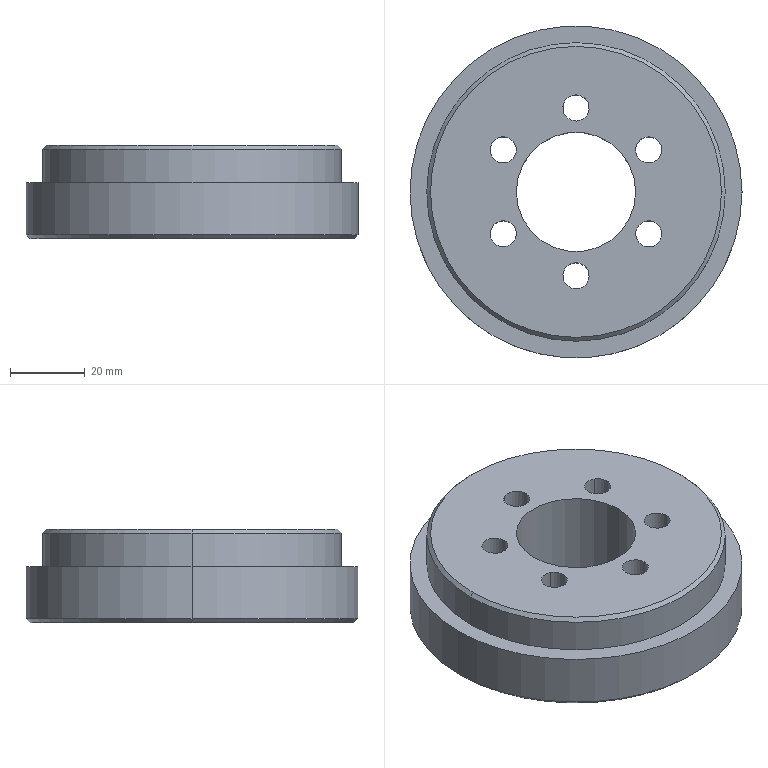Part | SolidWorks | features BaseBody 1 | 1 solid | 25 faces | box 89 x 89 x 25 mm | volume 117440 mm3 | cylinder 18 | cone 4 | plane 3 | commonest cylinder face diameters 7 x12 32 x2 80 x2 89 x2
STEP:
#1=CARTESIAN_POINT('',(17.736,8.219,0.));
#2=VERTEX_POINT('',#1);
#3=CARTESIAN_POINT('',(21.236,14.281,0.));
#4=VERTEX_POINT('',#3);
#5=CARTESIAN_POINT('',(19.486,11.25,0.));
#6=DIRECTION('',(0.,0.,1.));
#7=DIRECTION('',(0.5,0.866,0.));
#8=AXIS2_PLACEMENT_3D('',#5,#6,#7);
#9=CIRCLE('',#8,3.5);
#10=EDGE_CURVE('',#2,#4,#9,.T.);
#11=ORIENTED_EDGE('',*,*,#10,.F.);
#12=CARTESIAN_POINT('',(17.736,8.219,25.));
#13=VERTEX_POINT('',#12);
#14=CARTESIAN_POINT('',(17.736,8.219,0.));
#15=DIRECTION('',(0.,0.,1.));
#16=VECTOR('',#15,1000.);
#17=LINE('',#14,#16);
#18=EDGE_CURVE('',#2,#13,#17,.T.);
#19=ORIENTED_EDGE('',*,*,#18,.T.);
#20=CARTESIAN_POINT('',(21.236,14.281,25.));
#21=VERTEX_POINT('',#20);
#22=CARTESIAN_POINT('',(19.486,11.25,25.));
#23=DIRECTION('',(0.,0.,1.));
#24=DIRECTION('',(0.5,0.866,0.));
#25=AXIS2_PLACEMENT_3D('',#22,#23,#24);
#26=CIRCLE('',#25,3.5);
#27=EDGE_CURVE('',#13,#21,#26,.T.);
#28=ORIENTED_EDGE('',*,*,#27,.T.);
#29=CARTESIAN_POINT('',(21.236,14.281,0.));
#30=DIRECTION('',(0.,0.,1.));
#31=VECTOR('',#30,1000.);
#32=LINE('',#29,#31);
#33=EDGE_CURVE('',#4,#21,#32,.T.);
#34=ORIENTED_EDGE('',*,*,#33,.F.);
#35=EDGE_LOOP('',(#11,#19,#28,#34));
#36=FACE_OUTER_BOUND('',#35,.T.);
#37=CARTESIAN_POINT('',(19.486,11.25,0.));
#38=DIRECTION('',(0.,0.,1.));
#39=DIRECTION('',(0.5,0.866,0.));
#40=AXIS2_PLACEMENT_3D('',#37,#38,#39);
#41=CYLINDRICAL_SURFACE('',#40,3.5);
#42=ADVANCED_FACE('',(#36),#41,.F.);
#43=CARTESIAN_POINT('',(1.75,19.469,0.));
#44=VERTEX_POINT('',#43);
#45=CARTESIAN_POINT('',(-1.75,25.531,0.));
#46=VERTEX_POINT('',#45);
#47=CARTESIAN_POINT('',(0.,22.5,0.));
#48=DIRECTION('',(0.,0.,1.));
#49=DIRECTION('',(-0.5,0.866,0.));
#50=AXIS2_PLACEMENT_3D('',#47,#48,#49);
#51=CIRCLE('',#50,3.5);
#52=EDGE_CURVE('',#44,#46,#51,.T.);
#53=ORIENTED_EDGE('',*,*,#52,.F.);
#54=CARTESIAN_POINT('',(1.75,19.469,25.));
#55=VERTEX_POINT('',#54);
#56=CARTESIAN_POINT('',(1.75,19.469,0.));
#57=DIRECTION('',(0.,0.,1.));
#58=VECTOR('',#57,1000.);
#59=LINE('',#56,#58);
#60=EDGE_CURVE('',#44,#55,#59,.T.);
#61=ORIENTED_EDGE('',*,*,#60,.T.);
#62=CARTESIAN_POINT('',(-1.75,25.531,25.));
#63=VERTEX_POINT('',#62);
#64=CARTESIAN_POINT('',(0.,22.5,25.));
#65=DIRECTION('',(0.,0.,1.));
#66=DIRECTION('',(-0.5,0.866,0.));
#67=AXIS2_PLACEMENT_3D('',#64,#65,#66);
#68=CIRCLE('',#67,3.5);
#69=EDGE_CURVE('',#55,#63,#68,.T.);
#70=ORIENTED_EDGE('',*,*,#69,.T.);
#71=CARTESIAN_POINT('',(-1.75,25.531,0.));
#72=DIRECTION('',(0.,0.,1.));
#73=VECTOR('',#72,1000.);
#74=LINE('',#71,#73);
#75=EDGE_CURVE('',#46,#63,#74,.T.);
#76=ORIENTED_EDGE('',*,*,#75,.F.);
#77=EDGE_LOOP('',(#53,#61,#70,#76));
#78=FACE_OUTER_BOUND('',#77,.T.);
#79=CARTESIAN_POINT('',(0.,22.5,0.));
#80=DIRECTION('',(0.,0.,1.));
#81=DIRECTION('',(-0.5,0.866,0.));
#82=AXIS2_PLACEMENT_3D('',#79,#80,#81);
#83=CYLINDRICAL_SURFACE('',#82,3.5);
#84=ADVANCED_FACE('',(#78),#83,.F.);
#85=CARTESIAN_POINT('',(-15.986,11.25,0.));
#86=VERTEX_POINT('',#85);
#87=CARTESIAN_POINT('',(-22.986,11.25,0.));
#88=VERTEX_POINT('',#87);
#89=CARTESIAN_POINT('',(-19.486,11.25,0.));
#90=DIRECTION('',(0.,0.,1.));
#91=DIRECTION('',(-1.,0.,0.));
#92=AXIS2_PLACEMENT_3D('',#89,#90,#91);
#93=CIRCLE('',#92,3.5);
#94=EDGE_CURVE('',#86,#88,#93,.T.);
#95=ORIENTED_EDGE('',*,*,#94,.F.);
#96=CARTESIAN_POINT('',(-15.986,11.25,25.));
#97=VERTEX_POINT('',#96);
#98=CARTESIAN_POINT('',(-15.986,11.25,0.));
#99=DIRECTION('',(0.,0.,1.));
#100=VECTOR('',#99,1000.);
#101=LINE('',#98,#100);
#102=EDGE_CURVE('',#86,#97,#101,.T.);
#103=ORIENTED_EDGE('',*,*,#102,.T.);
#104=CARTESIAN_POINT('',(-22.986,11.25,25.));
#105=VERTEX_POINT('',#104);
#106=CARTESIAN_POINT('',(-19.486,11.25,25.));
#107=DIRECTION('',(0.,0.,1.));
#108=DIRECTION('',(-1.,0.,0.));
#109=AXIS2_PLACEMENT_3D('',#106,#107,#108);
#110=CIRCLE('',#109,3.5);
#111=EDGE_CURVE('',#97,#105,#110,.T.);
#112=ORIENTED_EDGE('',*,*,#111,.T.);
#113=CARTESIAN_POINT('',(-22.986,11.25,0.));
#114=DIRECTION('',(0.,0.,1.));
#115=VECTOR('',#114,1000.);
#116=LINE('',#113,#115);
#117=EDGE_CURVE('',#88,#105,#116,.T.);
#118=ORIENTED_EDGE('',*,*,#117,.F.);
#119=EDGE_LOOP('',(#95,#103,#112,#118));
#120=FACE_OUTER_BOUND('',#119,.T.);
#121=CARTESIAN_POINT('',(-19.486,11.25,0.));
#122=DIRECTION('',(0.,0.,1.));
#123=DIRECTION('',(-1.,0.,0.));
#124=AXIS2_PLACEMENT_3D('',#121,#122,#123);
#125=CYLINDRICAL_SURFACE('',#124,3.5);
#126=ADVANCED_FACE('',(#120),#125,.F.);
#127=CARTESIAN_POINT('',(-17.736,-8.219,0.));
#128=VERTEX_POINT('',#127);
#129=CARTESIAN_POINT('',(-21.236,-14.281,0.));
#130=VERTEX_POINT('',#129);
#131=CARTESIAN_POINT('',(-19.486,-11.25,0.));
#132=DIRECTION('',(0.,0.,1.));
#133=DIRECTION('',(-0.5,-0.866,0.));
#134=AXIS2_PLACEMENT_3D('',#131,#132,#133);
#135=CIRCLE('',#134,3.5);
#136=EDGE_CURVE('',#128,#130,#135,.T.);
#137=ORIENTED_EDGE('',*,*,#136,.F.);
#138=CARTESIAN_POINT('',(-17.736,-8.219,25.));
#139=VERTEX_POINT('',#138);
#140=CARTESIAN_POINT('',(-17.736,-8.219,0.));
#141=DIRECTION('',(0.,0.,1.));
#142=VECTOR('',#141,1000.);
#143=LINE('',#140,#142);
#144=EDGE_CURVE('',#128,#139,#143,.T.);
#145=ORIENTED_EDGE('',*,*,#144,.T.);
#146=CARTESIAN_POINT('',(-21.236,-14.281,25.));
#147=VERTEX_POINT('',#146);
#148=CARTESIAN_POINT('',(-19.486,-11.25,25.));
#149=DIRECTION('',(0.,0.,1.));
#150=DIRECTION('',(-0.5,-0.866,0.));
#151=AXIS2_PLACEMENT_3D('',#148,#149,#150);
#152=CIRCLE('',#151,3.5);
#153=EDGE_CURVE('',#139,#147,#152,.T.);
#154=ORIENTED_EDGE('',*,*,#153,.T.);
#155=CARTESIAN_POINT('',(-21.236,-14.281,0.));
#156=DIRECTION('',(0.,0.,1.));
#157=VECTOR('',#156,1000.);
#158=LINE('',#155,#157);
#159=EDGE_CURVE('',#130,#147,#158,.T.);
#160=ORIENTED_EDGE('',*,*,#159,.F.);
#161=EDGE_LOOP('',(#137,#145,#154,#160));
#162=FACE_OUTER_BOUND('',#161,.T.);
#163=CARTESIAN_POINT('',(-19.486,-11.25,0.));
#164=DIRECTION('',(0.,0.,1.));
#165=DIRECTION('',(-0.5,-0.866,0.));
#166=AXIS2_PLACEMENT_3D('',#163,#164,#165);
#167=CYLINDRICAL_SURFACE('',#166,3.5);
#168=ADVANCED_FACE('',(#162),#167,.F.);
#169=CARTESIAN_POINT('',(-1.75,-19.469,0.));
#170=VERTEX_POINT('',#169);
#171=CARTESIAN_POINT('',(1.75,-25.531,0.));
#172=VERTEX_POINT('',#171);
#173=CARTESIAN_POINT('',(0.,-22.5,0.));
#174=DIRECTION('',(0.,0.,1.));
#175=DIRECTION('',(0.5,-0.866,0.));
#176=AXIS2_PLACEMENT_3D('',#173,#174,#175);
#177=CIRCLE('',#176,3.5);
#178=EDGE_CURVE('',#170,#172,#177,.T.);
#179=ORIENTED_EDGE('',*,*,#178,.F.);
#180=CARTESIAN_POINT('',(-1.75,-19.469,25.));
#181=VERTEX_POINT('',#180);
#182=CARTESIAN_POINT('',(-1.75,-19.469,0.));
#183=DIRECTION('',(0.,0.,1.));
#184=VECTOR('',#183,1000.);
#185=LINE('',#182,#184);
#186=EDGE_CURVE('',#170,#181,#185,.T.);
#187=ORIENTED_EDGE('',*,*,#186,.T.);
#188=CARTESIAN_POINT('',(1.75,-25.531,25.));
#189=VERTEX_POINT('',#188);
#190=CARTESIAN_POINT('',(0.,-22.5,25.));
#191=DIRECTION('',(0.,0.,1.));
#192=DIRECTION('',(0.5,-0.866,0.));
#193=AXIS2_PLACEMENT_3D('',#190,#191,#192);
#194=CIRCLE('',#193,3.5);
#195=EDGE_CURVE('',#181,#189,#194,.T.);
#196=ORIENTED_EDGE('',*,*,#195,.T.);
#197=CARTESIAN_POINT('',(1.75,-25.531,0.));
#198=DIRECTION('',(0.,0.,1.));
#199=VECTOR('',#198,1000.);
#200=LINE('',#197,#199);
#201=EDGE_CURVE('',#172,#189,#200,.T.);
#202=ORIENTED_EDGE('',*,*,#201,.F.);
#203=EDGE_LOOP('',(#179,#187,#196,#202));
#204=FACE_OUTER_BOUND('',#203,.T.);
#205=CARTESIAN_POINT('',(0.,-22.5,0.));
#206=DIRECTION('',(0.,0.,1.));
#207=DIRECTION('',(0.5,-0.866,0.));
#208=AXIS2_PLACEMENT_3D('',#205,#206,#207);
#209=CYLINDRICAL_SURFACE('',#208,3.5);
#210=ADVANCED_FACE('',(#204),#209,.F.);
#211=CARTESIAN_POINT('',(15.986,-11.25,0.));
#212=VERTEX_POINT('',#211);
#213=CARTESIAN_POINT('',(22.986,-11.25,0.));
#214=VERTEX_POINT('',#213);
#215=CARTESIAN_POINT('',(19.486,-11.25,0.));
#216=DIRECTION('',(0.,0.,1.));
#217=DIRECTION('',(1.,0.,0.));
#218=AXIS2_PLACEMENT_3D('',#215,#216,#217);
#219=CIRCLE('',#218,3.5);
#220=EDGE_CURVE('',#212,#214,#219,.T.);
#221=ORIENTED_EDGE('',*,*,#220,.F.);
#222=CARTESIAN_POINT('',(15.986,-11.25,25.));
#223=VERTEX_POINT('',#222);
#224=CARTESIAN_POINT('',(15.986,-11.25,0.));
#225=DIRECTION('',(0.,0.,1.));
#226=VECTOR('',#225,1000.);
#227=LINE('',#224,#226);
#228=EDGE_CURVE('',#212,#223,#227,.T.);
#229=ORIENTED_EDGE('',*,*,#228,.T.);
#230=CARTESIAN_POINT('',(22.986,-11.25,25.));
#231=VERTEX_POINT('',#230);
#232=CARTESIAN_POINT('',(19.486,-11.25,25.));
#233=DIRECTION('',(0.,0.,1.));
#234=DIRECTION('',(1.,0.,0.));
#235=AXIS2_PLACEMENT_3D('',#232,#233,#234);
#236=CIRCLE('',#235,3.5);
#237=EDGE_CURVE('',#223,#231,#236,.T.);
#238=ORIENTED_EDGE('',*,*,#237,.T.);
#239=CARTESIAN_POINT('',(22.986,-11.25,0.));
#240=DIRECTION('',(0.,0.,1.));
#241=VECTOR('',#240,1000.);
#242=LINE('',#239,#241);
#243=EDGE_CURVE('',#214,#231,#242,.T.);
#244=ORIENTED_EDGE('',*,*,#243,.F.);
#245=EDGE_LOOP('',(#221,#229,#238,#244));
#246=FACE_OUTER_BOUND('',#245,.T.);
#247=CARTESIAN_POINT('',(19.486,-11.25,0.));
#248=DIRECTION('',(0.,0.,1.));
#249=DIRECTION('',(1.,0.,0.));
#250=AXIS2_PLACEMENT_3D('',#247,#248,#249);
#251=CYLINDRICAL_SURFACE('',#250,3.5);
#252=ADVANCED_FACE('',(#246),#251,.F.);
#253=CARTESIAN_POINT('',(-16.,0.,0.));
#254=VERTEX_POINT('',#253);
#255=CARTESIAN_POINT('',(16.,0.,0.));
#256=VERTEX_POINT('',#255);
#257=CARTESIAN_POINT('',(0.,0.,0.));
#258=DIRECTION('',(0.,0.,1.));
#259=DIRECTION('',(1.,0.,0.));
#260=AXIS2_PLACEMENT_3D('',#257,#258,#259);
#261=CIRCLE('',#260,16.);
#262=EDGE_CURVE('',#254,#256,#261,.T.);
#263=ORIENTED_EDGE('',*,*,#262,.F.);
#264=CARTESIAN_POINT('',(-16.,0.,25.));
#265=VERTEX_POINT('',#264);
#266=CARTESIAN_POINT('',(-16.,0.,0.));
#267=DIRECTION('',(0.,0.,1.));
#268=VECTOR('',#267,1000.);
#269=LINE('',#266,#268);
#270=EDGE_CURVE('',#254,#265,#269,.T.);
#271=ORIENTED_EDGE('',*,*,#270,.T.);
#272=CARTESIAN_POINT('',(16.,0.,25.));
#273=VERTEX_POINT('',#272);
#274=CARTESIAN_POINT('',(0.,0.,25.));
#275=DIRECTION('',(0.,0.,1.));
#276=DIRECTION('',(1.,0.,0.));
#277=AXIS2_PLACEMENT_3D('',#274,#275,#276);
#278=CIRCLE('',#277,16.);
#279=EDGE_CURVE('',#265,#273,#278,.T.);
#280=ORIENTED_EDGE('',*,*,#279,.T.);
#281=CARTESIAN_POINT('',(16.,0.,0.));
#282=DIRECTION('',(0.,0.,1.));
#283=VECTOR('',#282,1000.);
#284=LINE('',#281,#283);
#285=EDGE_CURVE('',#256,#273,#284,.T.);
#286=ORIENTED_EDGE('',*,*,#285,.F.);
#287=EDGE_LOOP('',(#263,#271,#280,#286));
#288=FACE_OUTER_BOUND('',#287,.T.);
#289=CARTESIAN_POINT('',(0.,0.,0.));
#290=DIRECTION('',(0.,0.,1.));
#291=DIRECTION('',(1.,0.,0.));
#292=AXIS2_PLACEMENT_3D('',#289,#290,#291);
#293=CYLINDRICAL_SURFACE('',#292,16.);
#294=ADVANCED_FACE('',(#288),#293,.F.);
#295=CARTESIAN_POINT('',(39.,0.,25.));
#296=VERTEX_POINT('',#295);
#297=CARTESIAN_POINT('',(-39.,0.,25.));
#298=VERTEX_POINT('',#297);
#299=CARTESIAN_POINT('',(0.,0.,25.));
#300=DIRECTION('',(0.,0.,1.));
#301=DIRECTION('',(1.,0.,0.));
#302=AXIS2_PLACEMENT_3D('',#299,#300,#301);
#303=CIRCLE('',#302,39.);
#304=EDGE_CURVE('',#296,#298,#303,.T.);
#305=ORIENTED_EDGE('',*,*,#304,.F.);
#306=CARTESIAN_POINT('',(40.,0.,24.));
#307=VERTEX_POINT('',#306);
#308=CARTESIAN_POINT('',(39.,0.,25.));
#309=DIRECTION('',(0.7071,0.,-0.7071));
#310=VECTOR('',#309,1000.);
#311=LINE('',#308,#310);
#312=EDGE_CURVE('',#296,#307,#311,.T.);
#313=ORIENTED_EDGE('',*,*,#312,.T.);
#314=CARTESIAN_POINT('',(-40.,0.,24.));
#315=VERTEX_POINT('',#314);
#316=CARTESIAN_POINT('',(0.,0.,24.));
#317=DIRECTION('',(0.,0.,-1.));
#318=DIRECTION('',(1.,0.,0.));
#319=AXIS2_PLACEMENT_3D('',#316,#317,#318);
#320=CIRCLE('',#319,40.);
#321=EDGE_CURVE('',#315,#307,#320,.T.);
#322=ORIENTED_EDGE('',*,*,#321,.F.);
#323=CARTESIAN_POINT('',(-39.,0.,25.));
#324=DIRECTION('',(-0.7071,0.,-0.7071));
#325=VECTOR('',#324,1000.);
#326=LINE('',#323,#325);
#327=EDGE_CURVE('',#298,#315,#326,.T.);
#328=ORIENTED_EDGE('',*,*,#327,.F.);
#329=EDGE_LOOP('',(#305,#313,#322,#328));
#330=FACE_OUTER_BOUND('',#329,.T.);
#331=CARTESIAN_POINT('',(0.,0.,25.));
#332=DIRECTION('',(0.,0.,-1.));
#333=DIRECTION('',(-1.,0.,0.));
#334=AXIS2_PLACEMENT_3D('',#331,#332,#333);
#335=CONICAL_SURFACE('',#334,39.,0.7854);
#336=ADVANCED_FACE('',(#330),#335,.T.);
#337=CARTESIAN_POINT('',(-43.5,0.,0.));
#338=VERTEX_POINT('',#337);
#339=CARTESIAN_POINT('',(43.5,0.,0.));
#340=VERTEX_POINT('',#339);
#341=CARTESIAN_POINT('',(0.,0.,0.));
#342=DIRECTION('',(0.,0.,-1.));
#343=DIRECTION('',(1.,0.,0.));
#344=AXIS2_PLACEMENT_3D('',#341,#342,#343);
#345=CIRCLE('',#344,43.5);
#346=EDGE_CURVE('',#338,#340,#345,.T.);
#347=ORIENTED_EDGE('',*,*,#346,.F.);
#348=CARTESIAN_POINT('',(-44.5,0.,1.));
#349=VERTEX_POINT('',#348);
#350=CARTESIAN_POINT('',(-44.5,0.,1.));
#351=DIRECTION('',(-0.7071,0.,0.7071));
#352=VECTOR('',#351,1000.);
#353=LINE('',#350,#352);
#354=EDGE_CURVE('',#338,#349,#353,.T.);
#355=ORIENTED_EDGE('',*,*,#354,.T.);
#356=CARTESIAN_POINT('',(44.5,0.,1.));
#357=VERTEX_POINT('',#356);
#358=CARTESIAN_POINT('',(0.,0.,1.));
#359=DIRECTION('',(0.,0.,1.));
#360=DIRECTION('',(1.,0.,0.));
#361=AXIS2_PLACEMENT_3D('',#358,#359,#360);
#362=CIRCLE('',#361,44.5);
#363=EDGE_CURVE('',#357,#349,#362,.T.);
#364=ORIENTED_EDGE('',*,*,#363,.F.);
#365=CARTESIAN_POINT('',(44.5,0.,1.));
#366=DIRECTION('',(0.7071,0.,0.7071));
#367=VECTOR('',#366,1000.);
#368=LINE('',#365,#367);
#369=EDGE_CURVE('',#340,#357,#368,.T.);
#370=ORIENTED_EDGE('',*,*,#369,.F.);
#371=EDGE_LOOP('',(#347,#355,#364,#370));
#372=FACE_OUTER_BOUND('',#371,.T.);
#373=CARTESIAN_POINT('',(0.,0.,1.));
#374=DIRECTION('',(0.,0.,1.));
#375=DIRECTION('',(1.,0.,0.));
#376=AXIS2_PLACEMENT_3D('',#373,#374,#375);
#377=CONICAL_SURFACE('',#376,44.5,0.7854);
#378=ADVANCED_FACE('',(#372),#377,.T.);
#379=ORIENTED_EDGE('',*,*,#321,.T.);
#380=CARTESIAN_POINT('',(40.,0.,15.));
#381=VERTEX_POINT('',#380);
#382=CARTESIAN_POINT('',(40.,0.,25.));
#383=DIRECTION('',(0.,0.,-1.));
#384=VECTOR('',#383,1000.);
#385=LINE('',#382,#384);
#386=EDGE_CURVE('',#307,#381,#385,.T.);
#387=ORIENTED_EDGE('',*,*,#386,.T.);
#388=CARTESIAN_POINT('',(-40.,0.,15.));
#389=VERTEX_POINT('',#388);
#390=CARTESIAN_POINT('',(0.,0.,15.));
#391=DIRECTION('',(0.,0.,1.));
#392=DIRECTION('',(1.,0.,0.));
#393=AXIS2_PLACEMENT_3D('',#390,#391,#392);
#394=CIRCLE('',#393,40.);
#395=EDGE_CURVE('',#381,#389,#394,.T.);
#396=ORIENTED_EDGE('',*,*,#395,.T.);
#397=CARTESIAN_POINT('',(-40.,0.,25.));
#398=DIRECTION('',(0.,0.,-1.));
#399=VECTOR('',#398,1000.);
#400=LINE('',#397,#399);
#401=EDGE_CURVE('',#315,#389,#400,.T.);
#402=ORIENTED_EDGE('',*,*,#401,.F.);
#403=EDGE_LOOP('',(#379,#387,#396,#402));
#404=FACE_OUTER_BOUND('',#403,.T.);
#405=CARTESIAN_POINT('',(0.,0.,25.));
#406=DIRECTION('',(0.,0.,-1.));
#407=DIRECTION('',(-1.,0.,0.));
#408=AXIS2_PLACEMENT_3D('',#405,#406,#407);
#409=CYLINDRICAL_SURFACE('',#408,40.);
#410=ADVANCED_FACE('',(#404),#409,.T.);
#411=CARTESIAN_POINT('',(44.5,0.,15.));
#412=VERTEX_POINT('',#411);
#413=CARTESIAN_POINT('',(-44.5,0.,15.));
#414=VERTEX_POINT('',#413);
#415=CARTESIAN_POINT('',(0.,0.,15.));
#416=DIRECTION('',(0.,0.,1.));
#417=DIRECTION('',(1.,0.,0.));
#418=AXIS2_PLACEMENT_3D('',#415,#416,#417);
#419=CIRCLE('',#418,44.5);
#420=EDGE_CURVE('',#412,#414,#419,.T.);
#421=ORIENTED_EDGE('',*,*,#420,.F.);
#422=CARTESIAN_POINT('',(44.5,0.,15.));
#423=DIRECTION('',(0.,0.,-1.));
#424=VECTOR('',#423,1000.);
#425=LINE('',#422,#424);
#426=EDGE_CURVE('',#412,#357,#425,.T.);
#427=ORIENTED_EDGE('',*,*,#426,.T.);
#428=ORIENTED_EDGE('',*,*,#363,.T.);
#429=CARTESIAN_POINT('',(-44.5,0.,15.));
#430=DIRECTION('',(0.,0.,-1.));
#431=VECTOR('',#430,1000.);
#432=LINE('',#429,#431);
#433=EDGE_CURVE('',#414,#349,#432,.T.);
#434=ORIENTED_EDGE('',*,*,#433,.F.);
#435=EDGE_LOOP('',(#421,#427,#428,#434));
#436=FACE_OUTER_BOUND('',#435,.T.);
#437=CARTESIAN_POINT('',(0.,0.,15.));
#438=DIRECTION('',(0.,0.,-1.));
#439=DIRECTION('',(-1.,0.,0.));
#440=AXIS2_PLACEMENT_3D('',#437,#438,#439);
#441=CYLINDRICAL_SURFACE('',#440,44.5);
#442=ADVANCED_FACE('',(#436),#441,.T.);
#443=ORIENTED_EDGE('',*,*,#426,.F.);
#444=CARTESIAN_POINT('',(0.,0.,15.));
#445=DIRECTION('',(0.,0.,1.));
#446=DIRECTION('',(1.,0.,0.));
#447=AXIS2_PLACEMENT_3D('',#444,#445,#446);
#448=CIRCLE('',#447,44.5);
#449=EDGE_CURVE('',#414,#412,#448,.T.);
#450=ORIENTED_EDGE('',*,*,#449,.F.);
#451=ORIENTED_EDGE('',*,*,#433,.T.);
#452=CARTESIAN_POINT('',(0.,0.,1.));
#453=DIRECTION('',(0.,0.,1.));
#454=DIRECTION('',(1.,0.,0.));
#455=AXIS2_PLACEMENT_3D('',#452,#453,#454);
#456=CIRCLE('',#455,44.5);
#457=EDGE_CURVE('',#349,#357,#456,.T.);
#458=ORIENTED_EDGE('',*,*,#457,.T.);
#459=EDGE_LOOP('',(#443,#450,#451,#458));
#460=FACE_OUTER_BOUND('',#459,.T.);
#461=CARTESIAN_POINT('',(0.,0.,15.));
#462=DIRECTION('',(0.,0.,-1.));
#463=DIRECTION('',(-1.,0.,0.));
#464=AXIS2_PLACEMENT_3D('',#461,#462,#463);
#465=CYLINDRICAL_SURFACE('',#464,44.5);
#466=ADVANCED_FACE('',(#460),#465,.T.);
#467=CARTESIAN_POINT('',(0.,0.,15.));
#468=DIRECTION('',(0.,0.,1.));
#469=DIRECTION('',(1.,0.,0.));
#470=AXIS2_PLACEMENT_3D('',#467,#468,#469);
#471=CIRCLE('',#470,40.);
#472=EDGE_CURVE('',#389,#381,#471,.T.);
#473=ORIENTED_EDGE('',*,*,#472,.F.);
#474=ORIENTED_EDGE('',*,*,#395,.F.);
#475=EDGE_LOOP('',(#473,#474));
#476=FACE_BOUND('',#475,.T.);
#477=ORIENTED_EDGE('',*,*,#449,.T.);
#478=ORIENTED_EDGE('',*,*,#420,.T.);
#479=EDGE_LOOP('',(#477,#478));
#480=FACE_OUTER_BOUND('',#479,.T.);
#481=CARTESIAN_POINT('',(0.,0.,15.));
#482=DIRECTION('',(0.,0.,1.));
#483=DIRECTION('',(1.,0.,0.));
#484=AXIS2_PLACEMENT_3D('',#481,#482,#483);
#485=PLANE('',#484);
#486=ADVANCED_FACE('',(#476,#480),#485,.T.);
#487=CARTESIAN_POINT('',(19.486,11.25,0.));
#488=DIRECTION('',(0.,0.,1.));
#489=DIRECTION('',(0.5,0.866,0.));
#490=AXIS2_PLACEMENT_3D('',#487,#488,#489);
#491=CIRCLE('',#490,3.5);
#492=EDGE_CURVE('',#4,#2,#491,.T.);
#493=ORIENTED_EDGE('',*,*,#492,.T.);
#494=ORIENTED_EDGE('',*,*,#10,.T.);
#495=EDGE_LOOP('',(#493,#494));
#496=FACE_BOUND('',#495,.T.);
#497=CARTESIAN_POINT('',(0.,22.5,0.));
#498=DIRECTION('',(0.,0.,1.));
#499=DIRECTION('',(-0.5,0.866,0.));
#500=AXIS2_PLACEMENT_3D('',#497,#498,#499);
#501=CIRCLE('',#500,3.5);
#502=EDGE_CURVE('',#46,#44,#501,.T.);
#503=ORIENTED_EDGE('',*,*,#502,.T.);
#504=ORIENTED_EDGE('',*,*,#52,.T.);
#505=EDGE_LOOP('',(#503,#504));
#506=FACE_BOUND('',#505,.T.);
#507=CARTESIAN_POINT('',(-19.486,11.25,0.));
#508=DIRECTION('',(0.,0.,1.));
#509=DIRECTION('',(-1.,0.,0.));
#510=AXIS2_PLACEMENT_3D('',#507,#508,#509);
#511=CIRCLE('',#510,3.5);
#512=EDGE_CURVE('',#88,#86,#511,.T.);
#513=ORIENTED_EDGE('',*,*,#512,.T.);
#514=ORIENTED_EDGE('',*,*,#94,.T.);
#515=EDGE_LOOP('',(#513,#514));
#516=FACE_BOUND('',#515,.T.);
#517=CARTESIAN_POINT('',(-19.486,-11.25,0.));
#518=DIRECTION('',(0.,0.,1.));
#519=DIRECTION('',(-0.5,-0.866,0.));
#520=AXIS2_PLACEMENT_3D('',#517,#518,#519);
#521=CIRCLE('',#520,3.5);
#522=EDGE_CURVE('',#130,#128,#521,.T.);
#523=ORIENTED_EDGE('',*,*,#522,.T.);
#524=ORIENTED_EDGE('',*,*,#136,.T.);
#525=EDGE_LOOP('',(#523,#524));
#526=FACE_BOUND('',#525,.T.);
#527=CARTESIAN_POINT('',(0.,-22.5,0.));
#528=DIRECTION('',(0.,0.,1.));
#529=DIRECTION('',(0.5,-0.866,0.));
#530=AXIS2_PLACEMENT_3D('',#527,#528,#529);
#531=CIRCLE('',#530,3.5);
#532=EDGE_CURVE('',#172,#170,#531,.T.);
#533=ORIENTED_EDGE('',*,*,#532,.T.);
#534=ORIENTED_EDGE('',*,*,#178,.T.);
#535=EDGE_LOOP('',(#533,#534));
#536=FACE_BOUND('',#535,.T.);
#537=CARTESIAN_POINT('',(19.486,-11.25,0.));
#538=DIRECTION('',(0.,0.,1.));
#539=DIRECTION('',(1.,0.,0.));
#540=AXIS2_PLACEMENT_3D('',#537,#538,#539);
#541=CIRCLE('',#540,3.5);
#542=EDGE_CURVE('',#214,#212,#541,.T.);
#543=ORIENTED_EDGE('',*,*,#542,.T.);
#544=ORIENTED_EDGE('',*,*,#220,.T.);
#545=EDGE_LOOP('',(#543,#544));
#546=FACE_BOUND('',#545,.T.);
#547=CARTESIAN_POINT('',(0.,0.,0.));
#548=DIRECTION('',(0.,0.,1.));
#549=DIRECTION('',(1.,0.,0.));
#550=AXIS2_PLACEMENT_3D('',#547,#548,#549);
#551=CIRCLE('',#550,16.);
#552=EDGE_CURVE('',#256,#254,#551,.T.);
#553=ORIENTED_EDGE('',*,*,#552,.T.);
#554=ORIENTED_EDGE('',*,*,#262,.T.);
#555=EDGE_LOOP('',(#553,#554));
#556=FACE_BOUND('',#555,.T.);
#557=CARTESIAN_POINT('',(0.,0.,0.));
#558=DIRECTION('',(0.,0.,-1.));
#559=DIRECTION('',(1.,0.,0.));
#560=AXIS2_PLACEMENT_3D('',#557,#558,#559);
#561=CIRCLE('',#560,43.5);
#562=EDGE_CURVE('',#340,#338,#561,.T.);
#563=ORIENTED_EDGE('',*,*,#562,.T.);
#564=ORIENTED_EDGE('',*,*,#346,.T.);
#565=EDGE_LOOP('',(#563,#564));
#566=FACE_OUTER_BOUND('',#565,.T.);
#567=CARTESIAN_POINT('',(0.,0.,0.));
#568=DIRECTION('',(0.,0.,1.));
#569=DIRECTION('',(1.,0.,0.));
#570=AXIS2_PLACEMENT_3D('',#567,#568,#569);
#571=PLANE('',#570);
#572=ADVANCED_FACE('',(#496,#506,#516,#526,#536,#546,#556,#566),#571,.F.);
#573=ORIENTED_EDGE('',*,*,#386,.F.);
#574=CARTESIAN_POINT('',(0.,0.,24.));
#575=DIRECTION('',(0.,0.,-1.));
#576=DIRECTION('',(1.,0.,0.));
#577=AXIS2_PLACEMENT_3D('',#574,#575,#576);
#578=CIRCLE('',#577,40.);
#579=EDGE_CURVE('',#307,#315,#578,.T.);
#580=ORIENTED_EDGE('',*,*,#579,.T.);
#581=ORIENTED_EDGE('',*,*,#401,.T.);
#582=ORIENTED_EDGE('',*,*,#472,.T.);
#583=EDGE_LOOP('',(#573,#580,#581,#582));
#584=FACE_OUTER_BOUND('',#583,.T.);
#585=CARTESIAN_POINT('',(0.,0.,25.));
#586=DIRECTION('',(0.,0.,-1.));
#587=DIRECTION('',(-1.,0.,0.));
#588=AXIS2_PLACEMENT_3D('',#585,#586,#587);
#589=CYLINDRICAL_SURFACE('',#588,40.);
#590=ADVANCED_FACE('',(#584),#589,.T.);
#591=CARTESIAN_POINT('',(19.486,11.25,25.));
#592=DIRECTION('',(0.,0.,1.));
#593=DIRECTION('',(0.5,0.866,0.));
#594=AXIS2_PLACEMENT_3D('',#591,#592,#593);
#595=CIRCLE('',#594,3.5);
#596=EDGE_CURVE('',#21,#13,#595,.T.);
#597=ORIENTED_EDGE('',*,*,#596,.F.);
#598=ORIENTED_EDGE('',*,*,#27,.F.);
#599=EDGE_LOOP('',(#597,#598));
#600=FACE_BOUND('',#599,.T.);
#601=CARTESIAN_POINT('',(0.,22.5,25.));
#602=DIRECTION('',(0.,0.,1.));
#603=DIRECTION('',(-0.5,0.866,0.));
#604=AXIS2_PLACEMENT_3D('',#601,#602,#603);
#605=CIRCLE('',#604,3.5);
#606=EDGE_CURVE('',#63,#55,#605,.T.);
#607=ORIENTED_EDGE('',*,*,#606,.F.);
#608=ORIENTED_EDGE('',*,*,#69,.F.);
#609=EDGE_LOOP('',(#607,#608));
#610=FACE_BOUND('',#609,.T.);
#611=CARTESIAN_POINT('',(-19.486,11.25,25.));
#612=DIRECTION('',(0.,0.,1.));
#613=DIRECTION('',(-1.,0.,0.));
#614=AXIS2_PLACEMENT_3D('',#611,#612,#613);
#615=CIRCLE('',#614,3.5);
#616=EDGE_CURVE('',#105,#97,#615,.T.);
#617=ORIENTED_EDGE('',*,*,#616,.F.);
#618=ORIENTED_EDGE('',*,*,#111,.F.);
#619=EDGE_LOOP('',(#617,#618));
#620=FACE_BOUND('',#619,.T.);
#621=CARTESIAN_POINT('',(-19.486,-11.25,25.));
#622=DIRECTION('',(0.,0.,1.));
#623=DIRECTION('',(-0.5,-0.866,0.));
#624=AXIS2_PLACEMENT_3D('',#621,#622,#623);
#625=CIRCLE('',#624,3.5);
#626=EDGE_CURVE('',#147,#139,#625,.T.);
#627=ORIENTED_EDGE('',*,*,#626,.F.);
#628=ORIENTED_EDGE('',*,*,#153,.F.);
#629=EDGE_LOOP('',(#627,#628));
#630=FACE_BOUND('',#629,.T.);
#631=CARTESIAN_POINT('',(0.,-22.5,25.));
#632=DIRECTION('',(0.,0.,1.));
#633=DIRECTION('',(0.5,-0.866,0.));
#634=AXIS2_PLACEMENT_3D('',#631,#632,#633);
#635=CIRCLE('',#634,3.5);
#636=EDGE_CURVE('',#189,#181,#635,.T.);
#637=ORIENTED_EDGE('',*,*,#636,.F.);
#638=ORIENTED_EDGE('',*,*,#195,.F.);
#639=EDGE_LOOP('',(#637,#638));
#640=FACE_BOUND('',#639,.T.);
#641=CARTESIAN_POINT('',(19.486,-11.25,25.));
#642=DIRECTION('',(0.,0.,1.));
#643=DIRECTION('',(1.,0.,0.));
#644=AXIS2_PLACEMENT_3D('',#641,#642,#643);
#645=CIRCLE('',#644,3.5);
#646=EDGE_CURVE('',#231,#223,#645,.T.);
#647=ORIENTED_EDGE('',*,*,#646,.F.);
#648=ORIENTED_EDGE('',*,*,#237,.F.);
#649=EDGE_LOOP('',(#647,#648));
#650=FACE_BOUND('',#649,.T.);
#651=CARTESIAN_POINT('',(0.,0.,25.));
#652=DIRECTION('',(0.,0.,1.));
#653=DIRECTION('',(1.,0.,0.));
#654=AXIS2_PLACEMENT_3D('',#651,#652,#653);
#655=CIRCLE('',#654,16.);
#656=EDGE_CURVE('',#273,#265,#655,.T.);
#657=ORIENTED_EDGE('',*,*,#656,.F.);
#658=ORIENTED_EDGE('',*,*,#279,.F.);
#659=EDGE_LOOP('',(#657,#658));
#660=FACE_BOUND('',#659,.T.);
#661=CARTESIAN_POINT('',(0.,0.,25.));
#662=DIRECTION('',(0.,0.,1.));
#663=DIRECTION('',(1.,0.,0.));
#664=AXIS2_PLACEMENT_3D('',#661,#662,#663);
#665=CIRCLE('',#664,39.);
#666=EDGE_CURVE('',#298,#296,#665,.T.);
#667=ORIENTED_EDGE('',*,*,#666,.T.);
#668=ORIENTED_EDGE('',*,*,#304,.T.);
#669=EDGE_LOOP('',(#667,#668));
#670=FACE_OUTER_BOUND('',#669,.T.);
#671=CARTESIAN_POINT('',(0.,0.,25.));
#672=DIRECTION('',(0.,0.,1.));
#673=DIRECTION('',(1.,0.,0.));
#674=AXIS2_PLACEMENT_3D('',#671,#672,#673);
#675=PLANE('',#674);
#676=ADVANCED_FACE('',(#600,#610,#620,#630,#640,#650,#660,#670),#675,.T.);
#677=ORIENTED_EDGE('',*,*,#354,.F.);
#678=ORIENTED_EDGE('',*,*,#562,.F.);
#679=ORIENTED_EDGE('',*,*,#369,.T.);
#680=ORIENTED_EDGE('',*,*,#457,.F.);
#681=EDGE_LOOP('',(#677,#678,#679,#680));
#682=FACE_OUTER_BOUND('',#681,.T.);
#683=CARTESIAN_POINT('',(0.,0.,1.));
#684=DIRECTION('',(0.,0.,1.));
#685=DIRECTION('',(1.,0.,0.));
#686=AXIS2_PLACEMENT_3D('',#683,#684,#685);
#687=CONICAL_SURFACE('',#686,44.5,0.7854);
#688=ADVANCED_FACE('',(#682),#687,.T.);
#689=ORIENTED_EDGE('',*,*,#312,.F.);
#690=ORIENTED_EDGE('',*,*,#666,.F.);
#691=ORIENTED_EDGE('',*,*,#327,.T.);
#692=ORIENTED_EDGE('',*,*,#579,.F.);
#693=EDGE_LOOP('',(#689,#690,#691,#692));
#694=FACE_OUTER_BOUND('',#693,.T.);
#695=CARTESIAN_POINT('',(0.,0.,25.));
#696=DIRECTION('',(0.,0.,-1.));
#697=DIRECTION('',(-1.,0.,0.));
#698=AXIS2_PLACEMENT_3D('',#695,#696,#697);
#699=CONICAL_SURFACE('',#698,39.,0.7854);
#700=ADVANCED_FACE('',(#694),#699,.T.);
#701=ORIENTED_EDGE('',*,*,#270,.F.);
#702=ORIENTED_EDGE('',*,*,#552,.F.);
#703=ORIENTED_EDGE('',*,*,#285,.T.);
#704=ORIENTED_EDGE('',*,*,#656,.T.);
#705=EDGE_LOOP('',(#701,#702,#703,#704));
#706=FACE_OUTER_BOUND('',#705,.T.);
#707=CARTESIAN_POINT('',(0.,0.,0.));
#708=DIRECTION('',(0.,0.,1.));
#709=DIRECTION('',(1.,0.,0.));
#710=AXIS2_PLACEMENT_3D('',#707,#708,#709);
#711=CYLINDRICAL_SURFACE('',#710,16.);
#712=ADVANCED_FACE('',(#706),#711,.F.);
#713=ORIENTED_EDGE('',*,*,#228,.F.);
#714=ORIENTED_EDGE('',*,*,#542,.F.);
#715=ORIENTED_EDGE('',*,*,#243,.T.);
#716=ORIENTED_EDGE('',*,*,#646,.T.);
#717=EDGE_LOOP('',(#713,#714,#715,#716));
#718=FACE_OUTER_BOUND('',#717,.T.);
#719=CARTESIAN_POINT('',(19.486,-11.25,0.));
#720=DIRECTION('',(0.,0.,1.));
#721=DIRECTION('',(1.,0.,0.));
#722=AXIS2_PLACEMENT_3D('',#719,#720,#721);
#723=CYLINDRICAL_SURFACE('',#722,3.5);
#724=ADVANCED_FACE('',(#718),#723,.F.);
#725=ORIENTED_EDGE('',*,*,#186,.F.);
#726=ORIENTED_EDGE('',*,*,#532,.F.);
#727=ORIENTED_EDGE('',*,*,#201,.T.);
#728=ORIENTED_EDGE('',*,*,#636,.T.);
#729=EDGE_LOOP('',(#725,#726,#727,#728));
#730=FACE_OUTER_BOUND('',#729,.T.);
#731=CARTESIAN_POINT('',(0.,-22.5,0.));
#732=DIRECTION('',(0.,0.,1.));
#733=DIRECTION('',(0.5,-0.866,0.));
#734=AXIS2_PLACEMENT_3D('',#731,#732,#733);
#735=CYLINDRICAL_SURFACE('',#734,3.5);
#736=ADVANCED_FACE('',(#730),#735,.F.);
#737=ORIENTED_EDGE('',*,*,#144,.F.);
#738=ORIENTED_EDGE('',*,*,#522,.F.);
#739=ORIENTED_EDGE('',*,*,#159,.T.);
#740=ORIENTED_EDGE('',*,*,#626,.T.);
#741=EDGE_LOOP('',(#737,#738,#739,#740));
#742=FACE_OUTER_BOUND('',#741,.T.);
#743=CARTESIAN_POINT('',(-19.486,-11.25,0.));
#744=DIRECTION('',(0.,0.,1.));
#745=DIRECTION('',(-0.5,-0.866,0.));
#746=AXIS2_PLACEMENT_3D('',#743,#744,#745);
#747=CYLINDRICAL_SURFACE('',#746,3.5);
#748=ADVANCED_FACE('',(#742),#747,.F.);
#749=ORIENTED_EDGE('',*,*,#102,.F.);
#750=ORIENTED_EDGE('',*,*,#512,.F.);
#751=ORIENTED_EDGE('',*,*,#117,.T.);
#752=ORIENTED_EDGE('',*,*,#616,.T.);
#753=EDGE_LOOP('',(#749,#750,#751,#752));
#754=FACE_OUTER_BOUND('',#753,.T.);
#755=CARTESIAN_POINT('',(-19.486,11.25,0.));
#756=DIRECTION('',(0.,0.,1.));
#757=DIRECTION('',(-1.,0.,0.));
#758=AXIS2_PLACEMENT_3D('',#755,#756,#757);
#759=CYLINDRICAL_SURFACE('',#758,3.5);
#760=ADVANCED_FACE('',(#754),#759,.F.);
#761=ORIENTED_EDGE('',*,*,#60,.F.);
#762=ORIENTED_EDGE('',*,*,#502,.F.);
#763=ORIENTED_EDGE('',*,*,#75,.T.);
#764=ORIENTED_EDGE('',*,*,#606,.T.);
#765=EDGE_LOOP('',(#761,#762,#763,#764));
#766=FACE_OUTER_BOUND('',#765,.T.);
#767=CARTESIAN_POINT('',(0.,22.5,0.));
#768=DIRECTION('',(0.,0.,1.));
#769=DIRECTION('',(-0.5,0.866,0.));
#770=AXIS2_PLACEMENT_3D('',#767,#768,#769);
#771=CYLINDRICAL_SURFACE('',#770,3.5);
#772=ADVANCED_FACE('',(#766),#771,.F.);
#773=ORIENTED_EDGE('',*,*,#18,.F.);
#774=ORIENTED_EDGE('',*,*,#492,.F.);
#775=ORIENTED_EDGE('',*,*,#33,.T.);
#776=ORIENTED_EDGE('',*,*,#596,.T.);
#777=EDGE_LOOP('',(#773,#774,#775,#776));
#778=FACE_OUTER_BOUND('',#777,.T.);
#779=CARTESIAN_POINT('',(19.486,11.25,0.));
#780=DIRECTION('',(0.,0.,1.));
#781=DIRECTION('',(0.5,0.866,0.));
#782=AXIS2_PLACEMENT_3D('',#779,#780,#781);
#783=CYLINDRICAL_SURFACE('',#782,3.5);
#784=ADVANCED_FACE('',(#778),#783,.F.);
#785=CLOSED_SHELL('',(#42,#84,#126,#168,#210,#252,#294,#336,#378,#410,#442,#466,#486,#572,#590,#676,#688,#700,#712,#724,#736,#748,#760,#772,#784));
#786=MANIFOLD_SOLID_BREP('',#785);
#787=CARTESIAN_POINT('',(0.,0.,0.));
#788=DIRECTION('',(0.,0.,1.));
#789=DIRECTION('',(1.,0.,0.));
#790=AXIS2_PLACEMENT_3D('',#787,#788,#789);
#791=(LENGTH_UNIT()NAMED_UNIT(*)SI_UNIT(.MILLI.,.METRE.));
#792=UNCERTAINTY_MEASURE_WITH_UNIT(LENGTH_MEASURE(0.00001),#791,'','');
#793=(NAMED_UNIT(*)PLANE_ANGLE_UNIT()SI_UNIT($,.RADIAN.));
#794=(NAMED_UNIT(*)SI_UNIT($,.STERADIAN.)SOLID_ANGLE_UNIT());
#795=(GEOMETRIC_REPRESENTATION_CONTEXT(3)GLOBAL_UNCERTAINTY_ASSIGNED_CONTEXT((#792))GLOBAL_UNIT_ASSIGNED_CONTEXT((#791,#793,#794))REPRESENTATION_CONTEXT('',''));
#796=ADVANCED_BREP_SHAPE_REPRESENTATION('',(#786,#790),#795);